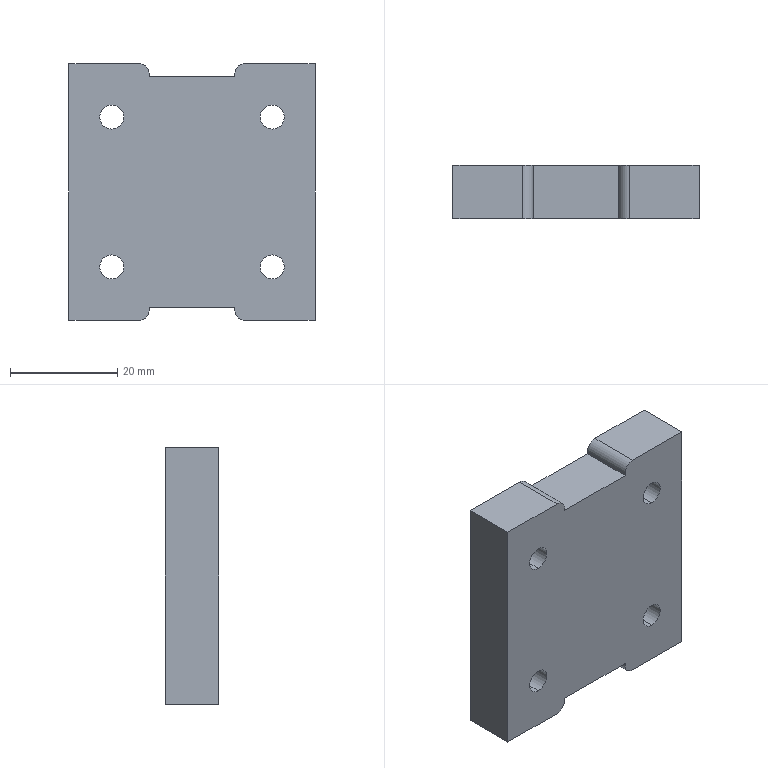Part | SolidWorks | features ICE 2, Extrusion 1, Fillet 1, HoleWzd 1 | 1 solid | 49 faces | box 46 x 10 x 48 mm | volume 19482 mm3 | cylinder 22 | plane 19 | cone 8 | commonest cylinder face diameters 4.5 x8 8 x8 4 x4 14 x2
STEP:
#1=CARTESIAN_POINT('',(0.,0.,17.));
#2=VERTEX_POINT('',#1);
#3=CARTESIAN_POINT('',(0.,0.,31.));
#4=VERTEX_POINT('',#3);
#5=CARTESIAN_POINT('',(0.,0.,24.));
#6=DIRECTION('',(0.,1.,0.));
#7=DIRECTION('',(0.,0.,1.));
#8=AXIS2_PLACEMENT_3D('',#5,#6,#7);
#9=CIRCLE('',#8,7.);
#10=EDGE_CURVE('',#2,#4,#9,.T.);
#11=ORIENTED_EDGE('',*,*,#10,.F.);
#12=CARTESIAN_POINT('',(0.,5.,17.));
#13=VERTEX_POINT('',#12);
#14=CARTESIAN_POINT('',(0.,0.,17.));
#15=DIRECTION('',(0.,1.,0.));
#16=VECTOR('',#15,1000.);
#17=LINE('',#14,#16);
#18=EDGE_CURVE('',#2,#13,#17,.T.);
#19=ORIENTED_EDGE('',*,*,#18,.T.);
#20=CARTESIAN_POINT('',(0.,5.,31.));
#21=VERTEX_POINT('',#20);
#22=CARTESIAN_POINT('',(0.,5.,24.));
#23=DIRECTION('',(0.,1.,0.));
#24=DIRECTION('',(0.,0.,1.));
#25=AXIS2_PLACEMENT_3D('',#22,#23,#24);
#26=CIRCLE('',#25,7.);
#27=EDGE_CURVE('',#13,#21,#26,.T.);
#28=ORIENTED_EDGE('',*,*,#27,.T.);
#29=CARTESIAN_POINT('',(0.,0.,31.));
#30=DIRECTION('',(0.,1.,0.));
#31=VECTOR('',#30,1000.);
#32=LINE('',#29,#31);
#33=EDGE_CURVE('',#4,#21,#32,.T.);
#34=ORIENTED_EDGE('',*,*,#33,.F.);
#35=EDGE_LOOP('',(#11,#19,#28,#34));
#36=FACE_OUTER_BOUND('',#35,.T.);
#37=CARTESIAN_POINT('',(0.,0.,24.));
#38=DIRECTION('',(0.,1.,0.));
#39=DIRECTION('',(0.,0.,1.));
#40=AXIS2_PLACEMENT_3D('',#37,#38,#39);
#41=CYLINDRICAL_SURFACE('',#40,7.);
#42=ADVANCED_FACE('',(#36),#41,.F.);
#43=CARTESIAN_POINT('',(-15.,4.975,6.));
#44=VERTEX_POINT('',#43);
#45=CARTESIAN_POINT('',(-15.,4.975,14.));
#46=VERTEX_POINT('',#45);
#47=CARTESIAN_POINT('',(-15.,4.975,10.));
#48=DIRECTION('',(0.,1.,0.));
#49=DIRECTION('',(0.,0.,1.));
#50=AXIS2_PLACEMENT_3D('',#47,#48,#49);
#51=CIRCLE('',#50,4.);
#52=EDGE_CURVE('',#44,#46,#51,.T.);
#53=ORIENTED_EDGE('',*,*,#52,.F.);
#54=CARTESIAN_POINT('',(-15.,5.,5.975));
#55=VERTEX_POINT('',#54);
#56=CARTESIAN_POINT('',(-15.,5.,5.975));
#57=DIRECTION('',(0.,0.7071,-0.7071));
#58=VECTOR('',#57,1000.);
#59=LINE('',#56,#58);
#60=EDGE_CURVE('',#44,#55,#59,.T.);
#61=ORIENTED_EDGE('',*,*,#60,.T.);
#62=CARTESIAN_POINT('',(-15.,5.,14.025));
#63=VERTEX_POINT('',#62);
#64=CARTESIAN_POINT('',(-15.,5.,10.));
#65=DIRECTION('',(0.,1.,0.));
#66=DIRECTION('',(0.,0.,1.));
#67=AXIS2_PLACEMENT_3D('',#64,#65,#66);
#68=CIRCLE('',#67,4.025);
#69=EDGE_CURVE('',#55,#63,#68,.T.);
#70=ORIENTED_EDGE('',*,*,#69,.T.);
#71=CARTESIAN_POINT('',(-15.,5.,14.025));
#72=DIRECTION('',(0.,0.7071,0.7071));
#73=VECTOR('',#72,1000.);
#74=LINE('',#71,#73);
#75=EDGE_CURVE('',#46,#63,#74,.T.);
#76=ORIENTED_EDGE('',*,*,#75,.F.);
#77=EDGE_LOOP('',(#53,#61,#70,#76));
#78=FACE_OUTER_BOUND('',#77,.T.);
#79=CARTESIAN_POINT('',(-15.,5.,10.));
#80=DIRECTION('',(0.,1.,0.));
#81=DIRECTION('',(0.,0.,1.));
#82=AXIS2_PLACEMENT_3D('',#79,#80,#81);
#83=CONICAL_SURFACE('',#82,4.025,0.7854);
#84=ADVANCED_FACE('',(#78),#83,.F.);
#85=CARTESIAN_POINT('',(-15.,2.4,6.));
#86=VERTEX_POINT('',#85);
#87=CARTESIAN_POINT('',(-15.,2.4,14.));
#88=VERTEX_POINT('',#87);
#89=CARTESIAN_POINT('',(-15.,2.4,10.));
#90=DIRECTION('',(0.,1.,0.));
#91=DIRECTION('',(0.,0.,1.));
#92=AXIS2_PLACEMENT_3D('',#89,#90,#91);
#93=CIRCLE('',#92,4.);
#94=EDGE_CURVE('',#86,#88,#93,.T.);
#95=ORIENTED_EDGE('',*,*,#94,.F.);
#96=CARTESIAN_POINT('',(-15.,5.,6.));
#97=DIRECTION('',(0.,1.,0.));
#98=VECTOR('',#97,1000.);
#99=LINE('',#96,#98);
#100=EDGE_CURVE('',#86,#44,#99,.T.);
#101=ORIENTED_EDGE('',*,*,#100,.T.);
#102=ORIENTED_EDGE('',*,*,#52,.T.);
#103=CARTESIAN_POINT('',(-15.,5.,14.));
#104=DIRECTION('',(0.,1.,0.));
#105=VECTOR('',#104,1000.);
#106=LINE('',#103,#105);
#107=EDGE_CURVE('',#88,#46,#106,.T.);
#108=ORIENTED_EDGE('',*,*,#107,.F.);
#109=EDGE_LOOP('',(#95,#101,#102,#108));
#110=FACE_OUTER_BOUND('',#109,.T.);
#111=CARTESIAN_POINT('',(-15.,5.,10.));
#112=DIRECTION('',(0.,1.,0.));
#113=DIRECTION('',(0.,0.,1.));
#114=AXIS2_PLACEMENT_3D('',#111,#112,#113);
#115=CYLINDRICAL_SURFACE('',#114,4.);
#116=ADVANCED_FACE('',(#110),#115,.F.);
#117=CARTESIAN_POINT('',(-15.,-5.,7.75));
#118=VERTEX_POINT('',#117);
#119=CARTESIAN_POINT('',(-15.,-5.,12.25));
#120=VERTEX_POINT('',#119);
#121=CARTESIAN_POINT('',(-15.,-5.,10.));
#122=DIRECTION('',(0.,1.,0.));
#123=DIRECTION('',(0.,0.,1.));
#124=AXIS2_PLACEMENT_3D('',#121,#122,#123);
#125=CIRCLE('',#124,2.25);
#126=EDGE_CURVE('',#118,#120,#125,.T.);
#127=ORIENTED_EDGE('',*,*,#126,.F.);
#128=CARTESIAN_POINT('',(-15.,2.4,7.75));
#129=VERTEX_POINT('',#128);
#130=CARTESIAN_POINT('',(-15.,5.,7.75));
#131=DIRECTION('',(0.,1.,0.));
#132=VECTOR('',#131,1000.);
#133=LINE('',#130,#132);
#134=EDGE_CURVE('',#118,#129,#133,.T.);
#135=ORIENTED_EDGE('',*,*,#134,.T.);
#136=CARTESIAN_POINT('',(-15.,2.4,12.25));
#137=VERTEX_POINT('',#136);
#138=CARTESIAN_POINT('',(-15.,2.4,10.));
#139=DIRECTION('',(0.,1.,0.));
#140=DIRECTION('',(0.,0.,1.));
#141=AXIS2_PLACEMENT_3D('',#138,#139,#140);
#142=CIRCLE('',#141,2.25);
#143=EDGE_CURVE('',#129,#137,#142,.T.);
#144=ORIENTED_EDGE('',*,*,#143,.T.);
#145=CARTESIAN_POINT('',(-15.,5.,12.25));
#146=DIRECTION('',(0.,1.,0.));
#147=VECTOR('',#146,1000.);
#148=LINE('',#145,#147);
#149=EDGE_CURVE('',#120,#137,#148,.T.);
#150=ORIENTED_EDGE('',*,*,#149,.F.);
#151=EDGE_LOOP('',(#127,#135,#144,#150));
#152=FACE_OUTER_BOUND('',#151,.T.);
#153=CARTESIAN_POINT('',(-15.,5.,10.));
#154=DIRECTION('',(0.,1.,0.));
#155=DIRECTION('',(0.,0.,1.));
#156=AXIS2_PLACEMENT_3D('',#153,#154,#155);
#157=CYLINDRICAL_SURFACE('',#156,2.25);
#158=ADVANCED_FACE('',(#152),#157,.F.);
#159=CARTESIAN_POINT('',(-15.,4.975,34.));
#160=VERTEX_POINT('',#159);
#161=CARTESIAN_POINT('',(-15.,4.975,42.));
#162=VERTEX_POINT('',#161);
#163=CARTESIAN_POINT('',(-15.,4.975,38.));
#164=DIRECTION('',(0.,1.,0.));
#165=DIRECTION('',(0.,0.,1.));
#166=AXIS2_PLACEMENT_3D('',#163,#164,#165);
#167=CIRCLE('',#166,4.);
#168=EDGE_CURVE('',#160,#162,#167,.T.);
#169=ORIENTED_EDGE('',*,*,#168,.F.);
#170=CARTESIAN_POINT('',(-15.,5.,33.975));
#171=VERTEX_POINT('',#170);
#172=CARTESIAN_POINT('',(-15.,5.,33.975));
#173=DIRECTION('',(0.,0.7071,-0.7071));
#174=VECTOR('',#173,1000.);
#175=LINE('',#172,#174);
#176=EDGE_CURVE('',#160,#171,#175,.T.);
#177=ORIENTED_EDGE('',*,*,#176,.T.);
#178=CARTESIAN_POINT('',(-15.,5.,42.025));
#179=VERTEX_POINT('',#178);
#180=CARTESIAN_POINT('',(-15.,5.,38.));
#181=DIRECTION('',(0.,1.,0.));
#182=DIRECTION('',(0.,0.,1.));
#183=AXIS2_PLACEMENT_3D('',#180,#181,#182);
#184=CIRCLE('',#183,4.025);
#185=EDGE_CURVE('',#171,#179,#184,.T.);
#186=ORIENTED_EDGE('',*,*,#185,.T.);
#187=CARTESIAN_POINT('',(-15.,5.,42.025));
#188=DIRECTION('',(0.,0.7071,0.7071));
#189=VECTOR('',#188,1000.);
#190=LINE('',#187,#189);
#191=EDGE_CURVE('',#162,#179,#190,.T.);
#192=ORIENTED_EDGE('',*,*,#191,.F.);
#193=EDGE_LOOP('',(#169,#177,#186,#192));
#194=FACE_OUTER_BOUND('',#193,.T.);
#195=CARTESIAN_POINT('',(-15.,5.,38.));
#196=DIRECTION('',(0.,1.,0.));
#197=DIRECTION('',(0.,0.,1.));
#198=AXIS2_PLACEMENT_3D('',#195,#196,#197);
#199=CONICAL_SURFACE('',#198,4.025,0.7854);
#200=ADVANCED_FACE('',(#194),#199,.F.);
#201=CARTESIAN_POINT('',(-15.,2.4,34.));
#202=VERTEX_POINT('',#201);
#203=CARTESIAN_POINT('',(-15.,2.4,42.));
#204=VERTEX_POINT('',#203);
#205=CARTESIAN_POINT('',(-15.,2.4,38.));
#206=DIRECTION('',(0.,1.,0.));
#207=DIRECTION('',(0.,0.,1.));
#208=AXIS2_PLACEMENT_3D('',#205,#206,#207);
#209=CIRCLE('',#208,4.);
#210=EDGE_CURVE('',#202,#204,#209,.T.);
#211=ORIENTED_EDGE('',*,*,#210,.F.);
#212=CARTESIAN_POINT('',(-15.,5.,34.));
#213=DIRECTION('',(0.,1.,0.));
#214=VECTOR('',#213,1000.);
#215=LINE('',#212,#214);
#216=EDGE_CURVE('',#202,#160,#215,.T.);
#217=ORIENTED_EDGE('',*,*,#216,.T.);
#218=ORIENTED_EDGE('',*,*,#168,.T.);
#219=CARTESIAN_POINT('',(-15.,5.,42.));
#220=DIRECTION('',(0.,1.,0.));
#221=VECTOR('',#220,1000.);
#222=LINE('',#219,#221);
#223=EDGE_CURVE('',#204,#162,#222,.T.);
#224=ORIENTED_EDGE('',*,*,#223,.F.);
#225=EDGE_LOOP('',(#211,#217,#218,#224));
#226=FACE_OUTER_BOUND('',#225,.T.);
#227=CARTESIAN_POINT('',(-15.,5.,38.));
#228=DIRECTION('',(0.,1.,0.));
#229=DIRECTION('',(0.,0.,1.));
#230=AXIS2_PLACEMENT_3D('',#227,#228,#229);
#231=CYLINDRICAL_SURFACE('',#230,4.);
#232=ADVANCED_FACE('',(#226),#231,.F.);
#233=CARTESIAN_POINT('',(-15.,-5.,35.75));
#234=VERTEX_POINT('',#233);
#235=CARTESIAN_POINT('',(-15.,-5.,40.25));
#236=VERTEX_POINT('',#235);
#237=CARTESIAN_POINT('',(-15.,-5.,38.));
#238=DIRECTION('',(0.,1.,0.));
#239=DIRECTION('',(0.,0.,1.));
#240=AXIS2_PLACEMENT_3D('',#237,#238,#239);
#241=CIRCLE('',#240,2.25);
#242=EDGE_CURVE('',#234,#236,#241,.T.);
#243=ORIENTED_EDGE('',*,*,#242,.F.);
#244=CARTESIAN_POINT('',(-15.,2.4,35.75));
#245=VERTEX_POINT('',#244);
#246=CARTESIAN_POINT('',(-15.,5.,35.75));
#247=DIRECTION('',(0.,1.,0.));
#248=VECTOR('',#247,1000.);
#249=LINE('',#246,#248);
#250=EDGE_CURVE('',#234,#245,#249,.T.);
#251=ORIENTED_EDGE('',*,*,#250,.T.);
#252=CARTESIAN_POINT('',(-15.,2.4,40.25));
#253=VERTEX_POINT('',#252);
#254=CARTESIAN_POINT('',(-15.,2.4,38.));
#255=DIRECTION('',(0.,1.,0.));
#256=DIRECTION('',(0.,0.,1.));
#257=AXIS2_PLACEMENT_3D('',#254,#255,#256);
#258=CIRCLE('',#257,2.25);
#259=EDGE_CURVE('',#245,#253,#258,.T.);
#260=ORIENTED_EDGE('',*,*,#259,.T.);
#261=CARTESIAN_POINT('',(-15.,5.,40.25));
#262=DIRECTION('',(0.,1.,0.));
#263=VECTOR('',#262,1000.);
#264=LINE('',#261,#263);
#265=EDGE_CURVE('',#236,#253,#264,.T.);
#266=ORIENTED_EDGE('',*,*,#265,.F.);
#267=EDGE_LOOP('',(#243,#251,#260,#266));
#268=FACE_OUTER_BOUND('',#267,.T.);
#269=CARTESIAN_POINT('',(-15.,5.,38.));
#270=DIRECTION('',(0.,1.,0.));
#271=DIRECTION('',(0.,0.,1.));
#272=AXIS2_PLACEMENT_3D('',#269,#270,#271);
#273=CYLINDRICAL_SURFACE('',#272,2.25);
#274=ADVANCED_FACE('',(#268),#273,.F.);
#275=CARTESIAN_POINT('',(15.,4.975,34.));
#276=VERTEX_POINT('',#275);
#277=CARTESIAN_POINT('',(15.,4.975,42.));
#278=VERTEX_POINT('',#277);
#279=CARTESIAN_POINT('',(15.,4.975,38.));
#280=DIRECTION('',(0.,1.,0.));
#281=DIRECTION('',(0.,0.,1.));
#282=AXIS2_PLACEMENT_3D('',#279,#280,#281);
#283=CIRCLE('',#282,4.);
#284=EDGE_CURVE('',#276,#278,#283,.T.);
#285=ORIENTED_EDGE('',*,*,#284,.F.);
#286=CARTESIAN_POINT('',(15.,5.,33.975));
#287=VERTEX_POINT('',#286);
#288=CARTESIAN_POINT('',(15.,5.,33.975));
#289=DIRECTION('',(0.,0.7071,-0.7071));
#290=VECTOR('',#289,1000.);
#291=LINE('',#288,#290);
#292=EDGE_CURVE('',#276,#287,#291,.T.);
#293=ORIENTED_EDGE('',*,*,#292,.T.);
#294=CARTESIAN_POINT('',(15.,5.,42.025));
#295=VERTEX_POINT('',#294);
#296=CARTESIAN_POINT('',(15.,5.,38.));
#297=DIRECTION('',(0.,1.,0.));
#298=DIRECTION('',(0.,0.,1.));
#299=AXIS2_PLACEMENT_3D('',#296,#297,#298);
#300=CIRCLE('',#299,4.025);
#301=EDGE_CURVE('',#287,#295,#300,.T.);
#302=ORIENTED_EDGE('',*,*,#301,.T.);
#303=CARTESIAN_POINT('',(15.,5.,42.025));
#304=DIRECTION('',(0.,0.7071,0.7071));
#305=VECTOR('',#304,1000.);
#306=LINE('',#303,#305);
#307=EDGE_CURVE('',#278,#295,#306,.T.);
#308=ORIENTED_EDGE('',*,*,#307,.F.);
#309=EDGE_LOOP('',(#285,#293,#302,#308));
#310=FACE_OUTER_BOUND('',#309,.T.);
#311=CARTESIAN_POINT('',(15.,5.,38.));
#312=DIRECTION('',(0.,1.,0.));
#313=DIRECTION('',(0.,0.,1.));
#314=AXIS2_PLACEMENT_3D('',#311,#312,#313);
#315=CONICAL_SURFACE('',#314,4.025,0.7854);
#316=ADVANCED_FACE('',(#310),#315,.F.);
#317=CARTESIAN_POINT('',(15.,2.4,34.));
#318=VERTEX_POINT('',#317);
#319=CARTESIAN_POINT('',(15.,2.4,42.));
#320=VERTEX_POINT('',#319);
#321=CARTESIAN_POINT('',(15.,2.4,38.));
#322=DIRECTION('',(0.,1.,0.));
#323=DIRECTION('',(0.,0.,1.));
#324=AXIS2_PLACEMENT_3D('',#321,#322,#323);
#325=CIRCLE('',#324,4.);
#326=EDGE_CURVE('',#318,#320,#325,.T.);
#327=ORIENTED_EDGE('',*,*,#326,.F.);
#328=CARTESIAN_POINT('',(15.,5.,34.));
#329=DIRECTION('',(0.,1.,0.));
#330=VECTOR('',#329,1000.);
#331=LINE('',#328,#330);
#332=EDGE_CURVE('',#318,#276,#331,.T.);
#333=ORIENTED_EDGE('',*,*,#332,.T.);
#334=ORIENTED_EDGE('',*,*,#284,.T.);
#335=CARTESIAN_POINT('',(15.,5.,42.));
#336=DIRECTION('',(0.,1.,0.));
#337=VECTOR('',#336,1000.);
#338=LINE('',#335,#337);
#339=EDGE_CURVE('',#320,#278,#338,.T.);
#340=ORIENTED_EDGE('',*,*,#339,.F.);
#341=EDGE_LOOP('',(#327,#333,#334,#340));
#342=FACE_OUTER_BOUND('',#341,.T.);
#343=CARTESIAN_POINT('',(15.,5.,38.));
#344=DIRECTION('',(0.,1.,0.));
#345=DIRECTION('',(0.,0.,1.));
#346=AXIS2_PLACEMENT_3D('',#343,#344,#345);
#347=CYLINDRICAL_SURFACE('',#346,4.);
#348=ADVANCED_FACE('',(#342),#347,.F.);
#349=CARTESIAN_POINT('',(15.,-5.,35.75));
#350=VERTEX_POINT('',#349);
#351=CARTESIAN_POINT('',(15.,-5.,40.25));
#352=VERTEX_POINT('',#351);
#353=CARTESIAN_POINT('',(15.,-5.,38.));
#354=DIRECTION('',(0.,1.,0.));
#355=DIRECTION('',(0.,0.,1.));
#356=AXIS2_PLACEMENT_3D('',#353,#354,#355);
#357=CIRCLE('',#356,2.25);
#358=EDGE_CURVE('',#350,#352,#357,.T.);
#359=ORIENTED_EDGE('',*,*,#358,.F.);
#360=CARTESIAN_POINT('',(15.,2.4,35.75));
#361=VERTEX_POINT('',#360);
#362=CARTESIAN_POINT('',(15.,5.,35.75));
#363=DIRECTION('',(0.,1.,0.));
#364=VECTOR('',#363,1000.);
#365=LINE('',#362,#364);
#366=EDGE_CURVE('',#350,#361,#365,.T.);
#367=ORIENTED_EDGE('',*,*,#366,.T.);
#368=CARTESIAN_POINT('',(15.,2.4,40.25));
#369=VERTEX_POINT('',#368);
#370=CARTESIAN_POINT('',(15.,2.4,38.));
#371=DIRECTION('',(0.,1.,0.));
#372=DIRECTION('',(0.,0.,1.));
#373=AXIS2_PLACEMENT_3D('',#370,#371,#372);
#374=CIRCLE('',#373,2.25);
#375=EDGE_CURVE('',#361,#369,#374,.T.);
#376=ORIENTED_EDGE('',*,*,#375,.T.);
#377=CARTESIAN_POINT('',(15.,5.,40.25));
#378=DIRECTION('',(0.,1.,0.));
#379=VECTOR('',#378,1000.);
#380=LINE('',#377,#379);
#381=EDGE_CURVE('',#352,#369,#380,.T.);
#382=ORIENTED_EDGE('',*,*,#381,.F.);
#383=EDGE_LOOP('',(#359,#367,#376,#382));
#384=FACE_OUTER_BOUND('',#383,.T.);
#385=CARTESIAN_POINT('',(15.,5.,38.));
#386=DIRECTION('',(0.,1.,0.));
#387=DIRECTION('',(0.,0.,1.));
#388=AXIS2_PLACEMENT_3D('',#385,#386,#387);
#389=CYLINDRICAL_SURFACE('',#388,2.25);
#390=ADVANCED_FACE('',(#384),#389,.F.);
#391=CARTESIAN_POINT('',(15.,4.975,6.));
#392=VERTEX_POINT('',#391);
#393=CARTESIAN_POINT('',(15.,4.975,14.));
#394=VERTEX_POINT('',#393);
#395=CARTESIAN_POINT('',(15.,4.975,10.));
#396=DIRECTION('',(0.,1.,0.));
#397=DIRECTION('',(0.,0.,1.));
#398=AXIS2_PLACEMENT_3D('',#395,#396,#397);
#399=CIRCLE('',#398,4.);
#400=EDGE_CURVE('',#392,#394,#399,.T.);
#401=ORIENTED_EDGE('',*,*,#400,.F.);
#402=CARTESIAN_POINT('',(15.,5.,5.975));
#403=VERTEX_POINT('',#402);
#404=CARTESIAN_POINT('',(15.,5.,5.975));
#405=DIRECTION('',(0.,0.7071,-0.7071));
#406=VECTOR('',#405,1000.);
#407=LINE('',#404,#406);
#408=EDGE_CURVE('',#392,#403,#407,.T.);
#409=ORIENTED_EDGE('',*,*,#408,.T.);
#410=CARTESIAN_POINT('',(15.,5.,14.025));
#411=VERTEX_POINT('',#410);
#412=CARTESIAN_POINT('',(15.,5.,10.));
#413=DIRECTION('',(0.,1.,0.));
#414=DIRECTION('',(0.,0.,1.));
#415=AXIS2_PLACEMENT_3D('',#412,#413,#414);
#416=CIRCLE('',#415,4.025);
#417=EDGE_CURVE('',#403,#411,#416,.T.);
#418=ORIENTED_EDGE('',*,*,#417,.T.);
#419=CARTESIAN_POINT('',(15.,5.,14.025));
#420=DIRECTION('',(0.,0.7071,0.7071));
#421=VECTOR('',#420,1000.);
#422=LINE('',#419,#421);
#423=EDGE_CURVE('',#394,#411,#422,.T.);
#424=ORIENTED_EDGE('',*,*,#423,.F.);
#425=EDGE_LOOP('',(#401,#409,#418,#424));
#426=FACE_OUTER_BOUND('',#425,.T.);
#427=CARTESIAN_POINT('',(15.,5.,10.));
#428=DIRECTION('',(0.,1.,0.));
#429=DIRECTION('',(0.,0.,1.));
#430=AXIS2_PLACEMENT_3D('',#427,#428,#429);
#431=CONICAL_SURFACE('',#430,4.025,0.7854);
#432=ADVANCED_FACE('',(#426),#431,.F.);
#433=CARTESIAN_POINT('',(15.,2.4,6.));
#434=VERTEX_POINT('',#433);
#435=CARTESIAN_POINT('',(15.,2.4,14.));
#436=VERTEX_POINT('',#435);
#437=CARTESIAN_POINT('',(15.,2.4,10.));
#438=DIRECTION('',(0.,1.,0.));
#439=DIRECTION('',(0.,0.,1.));
#440=AXIS2_PLACEMENT_3D('',#437,#438,#439);
#441=CIRCLE('',#440,4.);
#442=EDGE_CURVE('',#434,#436,#441,.T.);
#443=ORIENTED_EDGE('',*,*,#442,.F.);
#444=CARTESIAN_POINT('',(15.,5.,6.));
#445=DIRECTION('',(0.,1.,0.));
#446=VECTOR('',#445,1000.);
#447=LINE('',#444,#446);
#448=EDGE_CURVE('',#434,#392,#447,.T.);
#449=ORIENTED_EDGE('',*,*,#448,.T.);
#450=ORIENTED_EDGE('',*,*,#400,.T.);
#451=CARTESIAN_POINT('',(15.,5.,14.));
#452=DIRECTION('',(0.,1.,0.));
#453=VECTOR('',#452,1000.);
#454=LINE('',#451,#453);
#455=EDGE_CURVE('',#436,#394,#454,.T.);
#456=ORIENTED_EDGE('',*,*,#455,.F.);
#457=EDGE_LOOP('',(#443,#449,#450,#456));
#458=FACE_OUTER_BOUND('',#457,.T.);
#459=CARTESIAN_POINT('',(15.,5.,10.));
#460=DIRECTION('',(0.,1.,0.));
#461=DIRECTION('',(0.,0.,1.));
#462=AXIS2_PLACEMENT_3D('',#459,#460,#461);
#463=CYLINDRICAL_SURFACE('',#462,4.);
#464=ADVANCED_FACE('',(#458),#463,.F.);
#465=CARTESIAN_POINT('',(15.,-5.,7.75));
#466=VERTEX_POINT('',#465);
#467=CARTESIAN_POINT('',(15.,-5.,12.25));
#468=VERTEX_POINT('',#467);
#469=CARTESIAN_POINT('',(15.,-5.,10.));
#470=DIRECTION('',(0.,1.,0.));
#471=DIRECTION('',(0.,0.,1.));
#472=AXIS2_PLACEMENT_3D('',#469,#470,#471);
#473=CIRCLE('',#472,2.25);
#474=EDGE_CURVE('',#466,#468,#473,.T.);
#475=ORIENTED_EDGE('',*,*,#474,.F.);
#476=CARTESIAN_POINT('',(15.,2.4,7.75));
#477=VERTEX_POINT('',#476);
#478=CARTESIAN_POINT('',(15.,5.,7.75));
#479=DIRECTION('',(0.,1.,0.));
#480=VECTOR('',#479,1000.);
#481=LINE('',#478,#480);
#482=EDGE_CURVE('',#466,#477,#481,.T.);
#483=ORIENTED_EDGE('',*,*,#482,.T.);
#484=CARTESIAN_POINT('',(15.,2.4,12.25));
#485=VERTEX_POINT('',#484);
#486=CARTESIAN_POINT('',(15.,2.4,10.));
#487=DIRECTION('',(0.,1.,0.));
#488=DIRECTION('',(0.,0.,1.));
#489=AXIS2_PLACEMENT_3D('',#486,#487,#488);
#490=CIRCLE('',#489,2.25);
#491=EDGE_CURVE('',#477,#485,#490,.T.);
#492=ORIENTED_EDGE('',*,*,#491,.T.);
#493=CARTESIAN_POINT('',(15.,5.,12.25));
#494=DIRECTION('',(0.,1.,0.));
#495=VECTOR('',#494,1000.);
#496=LINE('',#493,#495);
#497=EDGE_CURVE('',#468,#485,#496,.T.);
#498=ORIENTED_EDGE('',*,*,#497,.F.);
#499=EDGE_LOOP('',(#475,#483,#492,#498));
#500=FACE_OUTER_BOUND('',#499,.T.);
#501=CARTESIAN_POINT('',(15.,5.,10.));
#502=DIRECTION('',(0.,1.,0.));
#503=DIRECTION('',(0.,0.,1.));
#504=AXIS2_PLACEMENT_3D('',#501,#502,#503);
#505=CYLINDRICAL_SURFACE('',#504,2.25);
#506=ADVANCED_FACE('',(#500),#505,.F.);
#507=CARTESIAN_POINT('',(-23.,-5.,48.));
#508=VERTEX_POINT('',#507);
#509=CARTESIAN_POINT('',(-10.,-5.,48.));
#510=VERTEX_POINT('',#509);
#511=CARTESIAN_POINT('',(-23.,-5.,48.));
#512=DIRECTION('',(1.,0.,0.));
#513=VECTOR('',#512,1000.);
#514=LINE('',#511,#513);
#515=EDGE_CURVE('',#508,#510,#514,.T.);
#516=ORIENTED_EDGE('',*,*,#515,.T.);
#517=CARTESIAN_POINT('',(-10.,5.,48.));
#518=VERTEX_POINT('',#517);
#519=CARTESIAN_POINT('',(-10.,5.,48.));
#520=DIRECTION('',(0.,1.,0.));
#521=VECTOR('',#520,1000.);
#522=LINE('',#519,#521);
#523=EDGE_CURVE('',#510,#518,#522,.T.);
#524=ORIENTED_EDGE('',*,*,#523,.T.);
#525=CARTESIAN_POINT('',(-23.,5.,48.));
#526=VERTEX_POINT('',#525);
#527=CARTESIAN_POINT('',(-23.,5.,48.));
#528=DIRECTION('',(-1.,0.,0.));
#529=VECTOR('',#528,1000.);
#530=LINE('',#527,#529);
#531=EDGE_CURVE('',#518,#526,#530,.T.);
#532=ORIENTED_EDGE('',*,*,#531,.T.);
#533=CARTESIAN_POINT('',(-23.,5.,48.));
#534=DIRECTION('',(0.,-1.,0.));
#535=VECTOR('',#534,1000.);
#536=LINE('',#533,#535);
#537=EDGE_CURVE('',#526,#508,#536,.T.);
#538=ORIENTED_EDGE('',*,*,#537,.T.);
#539=EDGE_LOOP('',(#516,#524,#532,#538));
#540=FACE_OUTER_BOUND('',#539,.T.);
#541=CARTESIAN_POINT('',(0.,0.,48.));
#542=DIRECTION('',(0.,0.,1.));
#543=DIRECTION('',(1.,0.,0.));
#544=AXIS2_PLACEMENT_3D('',#541,#542,#543);
#545=PLANE('',#544);
#546=ADVANCED_FACE('',(#540),#545,.T.);
#547=CARTESIAN_POINT('',(10.,-5.,0.));
#548=VERTEX_POINT('',#547);
#549=CARTESIAN_POINT('',(23.,-5.,0.));
#550=VERTEX_POINT('',#549);
#551=CARTESIAN_POINT('',(-23.,-5.,0.));
#552=DIRECTION('',(1.,0.,0.));
#553=VECTOR('',#552,1000.);
#554=LINE('',#551,#553);
#555=EDGE_CURVE('',#548,#550,#554,.T.);
#556=ORIENTED_EDGE('',*,*,#555,.F.);
#557=CARTESIAN_POINT('',(10.,5.,0.));
#558=VERTEX_POINT('',#557);
#559=CARTESIAN_POINT('',(10.,0.,0.));
#560=DIRECTION('',(0.,1.,0.));
#561=VECTOR('',#560,1000.);
#562=LINE('',#559,#561);
#563=EDGE_CURVE('',#548,#558,#562,.T.);
#564=ORIENTED_EDGE('',*,*,#563,.T.);
#565=CARTESIAN_POINT('',(23.,5.,0.));
#566=VERTEX_POINT('',#565);
#567=CARTESIAN_POINT('',(-23.,5.,0.));
#568=DIRECTION('',(-1.,0.,0.));
#569=VECTOR('',#568,1000.);
#570=LINE('',#567,#569);
#571=EDGE_CURVE('',#566,#558,#570,.T.);
#572=ORIENTED_EDGE('',*,*,#571,.F.);
#573=CARTESIAN_POINT('',(23.,5.,0.));
#574=DIRECTION('',(0.,1.,0.));
#575=VECTOR('',#574,1000.);
#576=LINE('',#573,#575);
#577=EDGE_CURVE('',#550,#566,#576,.T.);
#578=ORIENTED_EDGE('',*,*,#577,.F.);
#579=EDGE_LOOP('',(#556,#564,#572,#578));
#580=FACE_OUTER_BOUND('',#579,.T.);
#581=CARTESIAN_POINT('',(0.,0.,0.));
#582=DIRECTION('',(0.,0.,1.));
#583=DIRECTION('',(1.,0.,0.));
#584=AXIS2_PLACEMENT_3D('',#581,#582,#583);
#585=PLANE('',#584);
#586=ADVANCED_FACE('',(#580),#585,.F.);
#587=ORIENTED_EDGE('',*,*,#577,.T.);
#588=CARTESIAN_POINT('',(23.,5.,48.));
#589=VERTEX_POINT('',#588);
#590=CARTESIAN_POINT('',(23.,5.,48.));
#591=DIRECTION('',(0.,0.,-1.));
#592=VECTOR('',#591,1000.);
#593=LINE('',#590,#592);
#594=EDGE_CURVE('',#589,#566,#593,.T.);
#595=ORIENTED_EDGE('',*,*,#594,.F.);
#596=CARTESIAN_POINT('',(23.,-5.,48.));
#597=VERTEX_POINT('',#596);
#598=CARTESIAN_POINT('',(23.,5.,48.));
#599=DIRECTION('',(0.,1.,0.));
#600=VECTOR('',#599,1000.);
#601=LINE('',#598,#600);
#602=EDGE_CURVE('',#597,#589,#601,.T.);
#603=ORIENTED_EDGE('',*,*,#602,.F.);
#604=CARTESIAN_POINT('',(23.,-5.,48.));
#605=DIRECTION('',(0.,0.,-1.));
#606=VECTOR('',#605,1000.);
#607=LINE('',#604,#606);
#608=EDGE_CURVE('',#597,#550,#607,.T.);
#609=ORIENTED_EDGE('',*,*,#608,.T.);
#610=EDGE_LOOP('',(#587,#595,#603,#609));
#611=FACE_OUTER_BOUND('',#610,.T.);
#612=CARTESIAN_POINT('',(23.,5.,48.));
#613=DIRECTION('',(-1.,0.,0.));
#614=DIRECTION('',(0.,0.,1.));
#615=AXIS2_PLACEMENT_3D('',#612,#613,#614);
#616=PLANE('',#615);
#617=ADVANCED_FACE('',(#611),#616,.F.);
#618=CARTESIAN_POINT('',(0.,5.,24.));
#619=DIRECTION('',(0.,1.,0.));
#620=DIRECTION('',(0.,0.,1.));
#621=AXIS2_PLACEMENT_3D('',#618,#619,#620);
#622=CIRCLE('',#621,7.);
#623=EDGE_CURVE('',#21,#13,#622,.T.);
#624=ORIENTED_EDGE('',*,*,#623,.F.);
#625=ORIENTED_EDGE('',*,*,#27,.F.);
#626=EDGE_LOOP('',(#624,#625));
#627=FACE_BOUND('',#626,.T.);
#628=CARTESIAN_POINT('',(-15.,5.,10.));
#629=DIRECTION('',(0.,1.,0.));
#630=DIRECTION('',(0.,0.,1.));
#631=AXIS2_PLACEMENT_3D('',#628,#629,#630);
#632=CIRCLE('',#631,4.025);
#633=EDGE_CURVE('',#63,#55,#632,.T.);
#634=ORIENTED_EDGE('',*,*,#633,.F.);
#635=ORIENTED_EDGE('',*,*,#69,.F.);
#636=EDGE_LOOP('',(#634,#635));
#637=FACE_BOUND('',#636,.T.);
#638=CARTESIAN_POINT('',(-15.,5.,38.));
#639=DIRECTION('',(0.,1.,0.));
#640=DIRECTION('',(0.,0.,1.));
#641=AXIS2_PLACEMENT_3D('',#638,#639,#640);
#642=CIRCLE('',#641,4.025);
#643=EDGE_CURVE('',#179,#171,#642,.T.);
#644=ORIENTED_EDGE('',*,*,#643,.F.);
#645=ORIENTED_EDGE('',*,*,#185,.F.);
#646=EDGE_LOOP('',(#644,#645));
#647=FACE_BOUND('',#646,.T.);
#648=CARTESIAN_POINT('',(15.,5.,38.));
#649=DIRECTION('',(0.,1.,0.));
#650=DIRECTION('',(0.,0.,1.));
#651=AXIS2_PLACEMENT_3D('',#648,#649,#650);
#652=CIRCLE('',#651,4.025);
#653=EDGE_CURVE('',#295,#287,#652,.T.);
#654=ORIENTED_EDGE('',*,*,#653,.F.);
#655=ORIENTED_EDGE('',*,*,#301,.F.);
#656=EDGE_LOOP('',(#654,#655));
#657=FACE_BOUND('',#656,.T.);
#658=CARTESIAN_POINT('',(15.,5.,10.));
#659=DIRECTION('',(0.,1.,0.));
#660=DIRECTION('',(0.,0.,1.));
#661=AXIS2_PLACEMENT_3D('',#658,#659,#660);
#662=CIRCLE('',#661,4.025);
#663=EDGE_CURVE('',#411,#403,#662,.T.);
#664=ORIENTED_EDGE('',*,*,#663,.F.);
#665=ORIENTED_EDGE('',*,*,#417,.F.);
#666=EDGE_LOOP('',(#664,#665));
#667=FACE_BOUND('',#666,.T.);
#668=CARTESIAN_POINT('',(8.,5.,46.));
#669=VERTEX_POINT('',#668);
#670=CARTESIAN_POINT('',(8.,5.,45.5));
#671=VERTEX_POINT('',#670);
#672=CARTESIAN_POINT('',(8.,5.,50.5));
#673=DIRECTION('',(0.,0.,-1.));
#674=VECTOR('',#673,1000.);
#675=LINE('',#672,#674);
#676=EDGE_CURVE('',#669,#671,#675,.T.);
#677=ORIENTED_EDGE('',*,*,#676,.F.);
#678=CARTESIAN_POINT('',(10.,5.,48.));
#679=VERTEX_POINT('',#678);
#680=CARTESIAN_POINT('',(10.,5.,46.));
#681=DIRECTION('',(0.,1.,0.));
#682=DIRECTION('',(0.,0.,-1.));
#683=AXIS2_PLACEMENT_3D('',#680,#681,#682);
#684=CIRCLE('',#683,2.);
#685=EDGE_CURVE('',#669,#679,#684,.T.);
#686=ORIENTED_EDGE('',*,*,#685,.T.);
#687=CARTESIAN_POINT('',(-23.,5.,48.));
#688=DIRECTION('',(-1.,0.,0.));
#689=VECTOR('',#688,1000.);
#690=LINE('',#687,#689);
#691=EDGE_CURVE('',#589,#679,#690,.T.);
#692=ORIENTED_EDGE('',*,*,#691,.F.);
#693=ORIENTED_EDGE('',*,*,#594,.T.);
#694=ORIENTED_EDGE('',*,*,#571,.T.);
#695=CARTESIAN_POINT('',(8.,5.,2.));
#696=VERTEX_POINT('',#695);
#697=CARTESIAN_POINT('',(10.,5.,2.));
#698=DIRECTION('',(0.,1.,0.));
#699=DIRECTION('',(0.,0.,-1.));
#700=AXIS2_PLACEMENT_3D('',#697,#698,#699);
#701=CIRCLE('',#700,2.);
#702=EDGE_CURVE('',#558,#696,#701,.T.);
#703=ORIENTED_EDGE('',*,*,#702,.T.);
#704=CARTESIAN_POINT('',(8.,5.,2.5));
#705=VERTEX_POINT('',#704);
#706=CARTESIAN_POINT('',(8.,5.,-2.5));
#707=DIRECTION('',(0.,0.,-1.));
#708=VECTOR('',#707,1000.);
#709=LINE('',#706,#708);
#710=EDGE_CURVE('',#705,#696,#709,.T.);
#711=ORIENTED_EDGE('',*,*,#710,.F.);
#712=CARTESIAN_POINT('',(-8.,5.,2.5));
#713=VERTEX_POINT('',#712);
#714=CARTESIAN_POINT('',(-8.,5.,2.5));
#715=DIRECTION('',(1.,0.,0.));
#716=VECTOR('',#715,1000.);
#717=LINE('',#714,#716);
#718=EDGE_CURVE('',#713,#705,#717,.T.);
#719=ORIENTED_EDGE('',*,*,#718,.F.);
#720=CARTESIAN_POINT('',(-8.,5.,2.));
#721=VERTEX_POINT('',#720);
#722=CARTESIAN_POINT('',(-8.,5.,-2.5));
#723=DIRECTION('',(0.,0.,1.));
#724=VECTOR('',#723,1000.);
#725=LINE('',#722,#724);
#726=EDGE_CURVE('',#721,#713,#725,.T.);
#727=ORIENTED_EDGE('',*,*,#726,.F.);
#728=CARTESIAN_POINT('',(-10.,5.,0.));
#729=VERTEX_POINT('',#728);
#730=CARTESIAN_POINT('',(-10.,5.,2.));
#731=DIRECTION('',(0.,1.,0.));
#732=DIRECTION('',(0.,0.,-1.));
#733=AXIS2_PLACEMENT_3D('',#730,#731,#732);
#734=CIRCLE('',#733,2.);
#735=EDGE_CURVE('',#721,#729,#734,.T.);
#736=ORIENTED_EDGE('',*,*,#735,.T.);
#737=CARTESIAN_POINT('',(-23.,5.,0.));
#738=VERTEX_POINT('',#737);
#739=CARTESIAN_POINT('',(-23.,5.,0.));
#740=DIRECTION('',(-1.,0.,0.));
#741=VECTOR('',#740,1000.);
#742=LINE('',#739,#741);
#743=EDGE_CURVE('',#729,#738,#742,.T.);
#744=ORIENTED_EDGE('',*,*,#743,.T.);
#745=CARTESIAN_POINT('',(-23.,5.,48.));
#746=DIRECTION('',(0.,0.,-1.));
#747=VECTOR('',#746,1000.);
#748=LINE('',#745,#747);
#749=EDGE_CURVE('',#526,#738,#748,.T.);
#750=ORIENTED_EDGE('',*,*,#749,.F.);
#751=ORIENTED_EDGE('',*,*,#531,.F.);
#752=CARTESIAN_POINT('',(-8.,5.,46.));
#753=VERTEX_POINT('',#752);
#754=CARTESIAN_POINT('',(-10.,5.,46.));
#755=DIRECTION('',(0.,1.,0.));
#756=DIRECTION('',(0.,0.,-1.));
#757=AXIS2_PLACEMENT_3D('',#754,#755,#756);
#758=CIRCLE('',#757,2.);
#759=EDGE_CURVE('',#518,#753,#758,.T.);
#760=ORIENTED_EDGE('',*,*,#759,.T.);
#761=CARTESIAN_POINT('',(-8.,5.,45.5));
#762=VERTEX_POINT('',#761);
#763=CARTESIAN_POINT('',(-8.,5.,50.5));
#764=DIRECTION('',(0.,0.,1.));
#765=VECTOR('',#764,1000.);
#766=LINE('',#763,#765);
#767=EDGE_CURVE('',#762,#753,#766,.T.);
#768=ORIENTED_EDGE('',*,*,#767,.F.);
#769=CARTESIAN_POINT('',(-8.,5.,45.5));
#770=DIRECTION('',(-1.,0.,0.));
#771=VECTOR('',#770,1000.);
#772=LINE('',#769,#771);
#773=EDGE_CURVE('',#671,#762,#772,.T.);
#774=ORIENTED_EDGE('',*,*,#773,.F.);
#775=EDGE_LOOP('',(#677,#686,#692,#693,#694,#703,#711,#719,#727,#736,#744,#750,#751,#760,#768,#774));
#776=FACE_OUTER_BOUND('',#775,.T.);
#777=CARTESIAN_POINT('',(-23.,5.,48.));
#778=DIRECTION('',(0.,-1.,0.));
#779=DIRECTION('',(0.,0.,-1.));
#780=AXIS2_PLACEMENT_3D('',#777,#778,#779);
#781=PLANE('',#780);
#782=ADVANCED_FACE('',(#627,#637,#647,#657,#667,#776),#781,.F.);
#783=CARTESIAN_POINT('',(-23.,-5.,0.));
#784=VERTEX_POINT('',#783);
#785=CARTESIAN_POINT('',(-23.,5.,0.));
#786=DIRECTION('',(0.,-1.,0.));
#787=VECTOR('',#786,1000.);
#788=LINE('',#785,#787);
#789=EDGE_CURVE('',#738,#784,#788,.T.);
#790=ORIENTED_EDGE('',*,*,#789,.T.);
#791=CARTESIAN_POINT('',(-23.,-5.,48.));
#792=DIRECTION('',(0.,0.,-1.));
#793=VECTOR('',#792,1000.);
#794=LINE('',#791,#793);
#795=EDGE_CURVE('',#508,#784,#794,.T.);
#796=ORIENTED_EDGE('',*,*,#795,.F.);
#797=ORIENTED_EDGE('',*,*,#537,.F.);
#798=ORIENTED_EDGE('',*,*,#749,.T.);
#799=EDGE_LOOP('',(#790,#796,#797,#798));
#800=FACE_OUTER_BOUND('',#799,.T.);
#801=CARTESIAN_POINT('',(-23.,5.,48.));
#802=DIRECTION('',(1.,0.,0.));
#803=DIRECTION('',(0.,0.,-1.));
#804=AXIS2_PLACEMENT_3D('',#801,#802,#803);
#805=PLANE('',#804);
#806=ADVANCED_FACE('',(#800),#805,.F.);
#807=CARTESIAN_POINT('',(-15.,-5.,10.));
#808=DIRECTION('',(0.,1.,0.));
#809=DIRECTION('',(0.,0.,1.));
#810=AXIS2_PLACEMENT_3D('',#807,#808,#809);
#811=CIRCLE('',#810,2.25);
#812=EDGE_CURVE('',#120,#118,#811,.T.);
#813=ORIENTED_EDGE('',*,*,#812,.T.);
#814=ORIENTED_EDGE('',*,*,#126,.T.);
#815=EDGE_LOOP('',(#813,#814));
#816=FACE_BOUND('',#815,.T.);
#817=CARTESIAN_POINT('',(-15.,-5.,38.));
#818=DIRECTION('',(0.,1.,0.));
#819=DIRECTION('',(0.,0.,1.));
#820=AXIS2_PLACEMENT_3D('',#817,#818,#819);
#821=CIRCLE('',#820,2.25);
#822=EDGE_CURVE('',#236,#234,#821,.T.);
#823=ORIENTED_EDGE('',*,*,#822,.T.);
#824=ORIENTED_EDGE('',*,*,#242,.T.);
#825=EDGE_LOOP('',(#823,#824));
#826=FACE_BOUND('',#825,.T.);
#827=CARTESIAN_POINT('',(15.,-5.,38.));
#828=DIRECTION('',(0.,1.,0.));
#829=DIRECTION('',(0.,0.,1.));
#830=AXIS2_PLACEMENT_3D('',#827,#828,#829);
#831=CIRCLE('',#830,2.25);
#832=EDGE_CURVE('',#352,#350,#831,.T.);
#833=ORIENTED_EDGE('',*,*,#832,.T.);
#834=ORIENTED_EDGE('',*,*,#358,.T.);
#835=EDGE_LOOP('',(#833,#834));
#836=FACE_BOUND('',#835,.T.);
#837=CARTESIAN_POINT('',(15.,-5.,10.));
#838=DIRECTION('',(0.,1.,0.));
#839=DIRECTION('',(0.,0.,1.));
#840=AXIS2_PLACEMENT_3D('',#837,#838,#839);
#841=CIRCLE('',#840,2.25);
#842=EDGE_CURVE('',#468,#466,#841,.T.);
#843=ORIENTED_EDGE('',*,*,#842,.T.);
#844=ORIENTED_EDGE('',*,*,#474,.T.);
#845=EDGE_LOOP('',(#843,#844));
#846=FACE_BOUND('',#845,.T.);
#847=CARTESIAN_POINT('',(10.,-5.,48.));
#848=VERTEX_POINT('',#847);
#849=CARTESIAN_POINT('',(-23.,-5.,48.));
#850=DIRECTION('',(1.,0.,0.));
#851=VECTOR('',#850,1000.);
#852=LINE('',#849,#851);
#853=EDGE_CURVE('',#848,#597,#852,.T.);
#854=ORIENTED_EDGE('',*,*,#853,.F.);
#855=CARTESIAN_POINT('',(8.,-5.,46.));
#856=VERTEX_POINT('',#855);
#857=CARTESIAN_POINT('',(10.,-5.,46.));
#858=DIRECTION('',(0.,-1.,0.));
#859=DIRECTION('',(0.,0.,1.));
#860=AXIS2_PLACEMENT_3D('',#857,#858,#859);
#861=CIRCLE('',#860,2.);
#862=EDGE_CURVE('',#848,#856,#861,.T.);
#863=ORIENTED_EDGE('',*,*,#862,.T.);
#864=CARTESIAN_POINT('',(8.,-5.,45.5));
#865=VERTEX_POINT('',#864);
#866=CARTESIAN_POINT('',(8.,-5.,50.5));
#867=DIRECTION('',(0.,0.,-1.));
#868=VECTOR('',#867,1000.);
#869=LINE('',#866,#868);
#870=EDGE_CURVE('',#856,#865,#869,.T.);
#871=ORIENTED_EDGE('',*,*,#870,.T.);
#872=CARTESIAN_POINT('',(-8.,-5.,45.5));
#873=VERTEX_POINT('',#872);
#874=CARTESIAN_POINT('',(-8.,-5.,45.5));
#875=DIRECTION('',(-1.,0.,0.));
#876=VECTOR('',#875,1000.);
#877=LINE('',#874,#876);
#878=EDGE_CURVE('',#865,#873,#877,.T.);
#879=ORIENTED_EDGE('',*,*,#878,.T.);
#880=CARTESIAN_POINT('',(-8.,-5.,46.));
#881=VERTEX_POINT('',#880);
#882=CARTESIAN_POINT('',(-8.,-5.,50.5));
#883=DIRECTION('',(0.,0.,1.));
#884=VECTOR('',#883,1000.);
#885=LINE('',#882,#884);
#886=EDGE_CURVE('',#873,#881,#885,.T.);
#887=ORIENTED_EDGE('',*,*,#886,.T.);
#888=CARTESIAN_POINT('',(-10.,-5.,46.));
#889=DIRECTION('',(0.,-1.,0.));
#890=DIRECTION('',(0.,0.,1.));
#891=AXIS2_PLACEMENT_3D('',#888,#889,#890);
#892=CIRCLE('',#891,2.);
#893=EDGE_CURVE('',#881,#510,#892,.T.);
#894=ORIENTED_EDGE('',*,*,#893,.T.);
#895=ORIENTED_EDGE('',*,*,#515,.F.);
#896=ORIENTED_EDGE('',*,*,#795,.T.);
#897=CARTESIAN_POINT('',(-10.,-5.,0.));
#898=VERTEX_POINT('',#897);
#899=CARTESIAN_POINT('',(-23.,-5.,0.));
#900=DIRECTION('',(1.,0.,0.));
#901=VECTOR('',#900,1000.);
#902=LINE('',#899,#901);
#903=EDGE_CURVE('',#784,#898,#902,.T.);
#904=ORIENTED_EDGE('',*,*,#903,.T.);
#905=CARTESIAN_POINT('',(-8.,-5.,2.));
#906=VERTEX_POINT('',#905);
#907=CARTESIAN_POINT('',(-10.,-5.,2.));
#908=DIRECTION('',(0.,-1.,0.));
#909=DIRECTION('',(0.,0.,1.));
#910=AXIS2_PLACEMENT_3D('',#907,#908,#909);
#911=CIRCLE('',#910,2.);
#912=EDGE_CURVE('',#898,#906,#911,.T.);
#913=ORIENTED_EDGE('',*,*,#912,.T.);
#914=CARTESIAN_POINT('',(-8.,-5.,2.5));
#915=VERTEX_POINT('',#914);
#916=CARTESIAN_POINT('',(-8.,-5.,-2.5));
#917=DIRECTION('',(0.,0.,1.));
#918=VECTOR('',#917,1000.);
#919=LINE('',#916,#918);
#920=EDGE_CURVE('',#906,#915,#919,.T.);
#921=ORIENTED_EDGE('',*,*,#920,.T.);
#922=CARTESIAN_POINT('',(8.,-5.,2.5));
#923=VERTEX_POINT('',#922);
#924=CARTESIAN_POINT('',(-8.,-5.,2.5));
#925=DIRECTION('',(1.,0.,0.));
#926=VECTOR('',#925,1000.);
#927=LINE('',#924,#926);
#928=EDGE_CURVE('',#915,#923,#927,.T.);
#929=ORIENTED_EDGE('',*,*,#928,.T.);
#930=CARTESIAN_POINT('',(8.,-5.,2.));
#931=VERTEX_POINT('',#930);
#932=CARTESIAN_POINT('',(8.,-5.,-2.5));
#933=DIRECTION('',(0.,0.,-1.));
#934=VECTOR('',#933,1000.);
#935=LINE('',#932,#934);
#936=EDGE_CURVE('',#923,#931,#935,.T.);
#937=ORIENTED_EDGE('',*,*,#936,.T.);
#938=CARTESIAN_POINT('',(10.,-5.,2.));
#939=DIRECTION('',(0.,-1.,0.));
#940=DIRECTION('',(0.,0.,1.));
#941=AXIS2_PLACEMENT_3D('',#938,#939,#940);
#942=CIRCLE('',#941,2.);
#943=EDGE_CURVE('',#931,#548,#942,.T.);
#944=ORIENTED_EDGE('',*,*,#943,.T.);
#945=ORIENTED_EDGE('',*,*,#555,.T.);
#946=ORIENTED_EDGE('',*,*,#608,.F.);
#947=EDGE_LOOP('',(#854,#863,#871,#879,#887,#894,#895,#896,#904,#913,#921,#929,#937,#944,#945,#946));
#948=FACE_OUTER_BOUND('',#947,.T.);
#949=CARTESIAN_POINT('',(-23.,-5.,48.));
#950=DIRECTION('',(0.,1.,0.));
#951=DIRECTION('',(0.,0.,1.));
#952=AXIS2_PLACEMENT_3D('',#949,#950,#951);
#953=PLANE('',#952);
#954=ADVANCED_FACE('',(#816,#826,#836,#846,#948),#953,.F.);
#955=ORIENTED_EDGE('',*,*,#691,.T.);
#956=CARTESIAN_POINT('',(10.,-5.,48.));
#957=DIRECTION('',(0.,-1.,0.));
#958=VECTOR('',#957,1000.);
#959=LINE('',#956,#958);
#960=EDGE_CURVE('',#679,#848,#959,.T.);
#961=ORIENTED_EDGE('',*,*,#960,.T.);
#962=ORIENTED_EDGE('',*,*,#853,.T.);
#963=ORIENTED_EDGE('',*,*,#602,.T.);
#964=EDGE_LOOP('',(#955,#961,#962,#963));
#965=FACE_OUTER_BOUND('',#964,.T.);
#966=CARTESIAN_POINT('',(0.,0.,48.));
#967=DIRECTION('',(0.,0.,1.));
#968=DIRECTION('',(1.,0.,0.));
#969=AXIS2_PLACEMENT_3D('',#966,#967,#968);
#970=PLANE('',#969);
#971=ADVANCED_FACE('',(#965),#970,.T.);
#972=ORIENTED_EDGE('',*,*,#743,.F.);
#973=CARTESIAN_POINT('',(-10.,0.,0.));
#974=DIRECTION('',(0.,-1.,0.));
#975=VECTOR('',#974,1000.);
#976=LINE('',#973,#975);
#977=EDGE_CURVE('',#729,#898,#976,.T.);
#978=ORIENTED_EDGE('',*,*,#977,.T.);
#979=ORIENTED_EDGE('',*,*,#903,.F.);
#980=ORIENTED_EDGE('',*,*,#789,.F.);
#981=EDGE_LOOP('',(#972,#978,#979,#980));
#982=FACE_OUTER_BOUND('',#981,.T.);
#983=CARTESIAN_POINT('',(0.,0.,0.));
#984=DIRECTION('',(0.,0.,1.));
#985=DIRECTION('',(1.,0.,0.));
#986=AXIS2_PLACEMENT_3D('',#983,#984,#985);
#987=PLANE('',#986);
#988=ADVANCED_FACE('',(#982),#987,.F.);
#989=ORIENTED_EDGE('',*,*,#710,.T.);
#990=CARTESIAN_POINT('',(8.,-5.,2.));
#991=DIRECTION('',(0.,-1.,0.));
#992=VECTOR('',#991,1000.);
#993=LINE('',#990,#992);
#994=EDGE_CURVE('',#696,#931,#993,.T.);
#995=ORIENTED_EDGE('',*,*,#994,.T.);
#996=ORIENTED_EDGE('',*,*,#936,.F.);
#997=CARTESIAN_POINT('',(8.,-5.,2.5));
#998=DIRECTION('',(0.,1.,0.));
#999=VECTOR('',#998,1000.);
#1000=LINE('',#997,#999);
#1001=EDGE_CURVE('',#923,#705,#1000,.T.);
#1002=ORIENTED_EDGE('',*,*,#1001,.T.);
#1003=EDGE_LOOP('',(#989,#995,#996,#1002));
#1004=FACE_OUTER_BOUND('',#1003,.T.);
#1005=CARTESIAN_POINT('',(8.,-5.,-2.5));
#1006=DIRECTION('',(1.,0.,0.));
#1007=DIRECTION('',(0.,0.,-1.));
#1008=AXIS2_PLACEMENT_3D('',#1005,#1006,#1007);
#1009=PLANE('',#1008);
#1010=ADVANCED_FACE('',(#1004),#1009,.F.);
#1011=ORIENTED_EDGE('',*,*,#920,.F.);
#1012=CARTESIAN_POINT('',(-8.,-5.,2.));
#1013=DIRECTION('',(0.,1.,0.));
#1014=VECTOR('',#1013,1000.);
#1015=LINE('',#1012,#1014);
#1016=EDGE_CURVE('',#906,#721,#1015,.T.);
#1017=ORIENTED_EDGE('',*,*,#1016,.T.);
#1018=ORIENTED_EDGE('',*,*,#726,.T.);
#1019=CARTESIAN_POINT('',(-8.,-5.,2.5));
#1020=DIRECTION('',(0.,1.,0.));
#1021=VECTOR('',#1020,1000.);
#1022=LINE('',#1019,#1021);
#1023=EDGE_CURVE('',#915,#713,#1022,.T.);
#1024=ORIENTED_EDGE('',*,*,#1023,.F.);
#1025=EDGE_LOOP('',(#1011,#1017,#1018,#1024));
#1026=FACE_OUTER_BOUND('',#1025,.T.);
#1027=CARTESIAN_POINT('',(-8.,-5.,-2.5));
#1028=DIRECTION('',(-1.,0.,0.));
#1029=DIRECTION('',(0.,0.,1.));
#1030=AXIS2_PLACEMENT_3D('',#1027,#1028,#1029);
#1031=PLANE('',#1030);
#1032=ADVANCED_FACE('',(#1026),#1031,.F.);
#1033=ORIENTED_EDGE('',*,*,#718,.T.);
#1034=ORIENTED_EDGE('',*,*,#1001,.F.);
#1035=ORIENTED_EDGE('',*,*,#928,.F.);
#1036=ORIENTED_EDGE('',*,*,#1023,.T.);
#1037=EDGE_LOOP('',(#1033,#1034,#1035,#1036));
#1038=FACE_OUTER_BOUND('',#1037,.T.);
#1039=CARTESIAN_POINT('',(-8.,-5.,2.5));
#1040=DIRECTION('',(0.,0.,1.));
#1041=DIRECTION('',(1.,0.,0.));
#1042=AXIS2_PLACEMENT_3D('',#1039,#1040,#1041);
#1043=PLANE('',#1042);
#1044=ADVANCED_FACE('',(#1038),#1043,.F.);
#1045=ORIENTED_EDGE('',*,*,#767,.T.);
#1046=CARTESIAN_POINT('',(-8.,-5.,46.));
#1047=DIRECTION('',(0.,-1.,0.));
#1048=VECTOR('',#1047,1000.);
#1049=LINE('',#1046,#1048);
#1050=EDGE_CURVE('',#753,#881,#1049,.T.);
#1051=ORIENTED_EDGE('',*,*,#1050,.T.);
#1052=ORIENTED_EDGE('',*,*,#886,.F.);
#1053=CARTESIAN_POINT('',(-8.,-5.,45.5));
#1054=DIRECTION('',(0.,1.,0.));
#1055=VECTOR('',#1054,1000.);
#1056=LINE('',#1053,#1055);
#1057=EDGE_CURVE('',#873,#762,#1056,.T.);
#1058=ORIENTED_EDGE('',*,*,#1057,.T.);
#1059=EDGE_LOOP('',(#1045,#1051,#1052,#1058));
#1060=FACE_OUTER_BOUND('',#1059,.T.);
#1061=CARTESIAN_POINT('',(-8.,-5.,50.5));
#1062=DIRECTION('',(-1.,0.,0.));
#1063=DIRECTION('',(0.,0.,1.));
#1064=AXIS2_PLACEMENT_3D('',#1061,#1062,#1063);
#1065=PLANE('',#1064);
#1066=ADVANCED_FACE('',(#1060),#1065,.F.);
#1067=ORIENTED_EDGE('',*,*,#773,.T.);
#1068=ORIENTED_EDGE('',*,*,#1057,.F.);
#1069=ORIENTED_EDGE('',*,*,#878,.F.);
#1070=CARTESIAN_POINT('',(8.,-5.,45.5));
#1071=DIRECTION('',(0.,1.,0.));
#1072=VECTOR('',#1071,1000.);
#1073=LINE('',#1070,#1072);
#1074=EDGE_CURVE('',#865,#671,#1073,.T.);
#1075=ORIENTED_EDGE('',*,*,#1074,.T.);
#1076=EDGE_LOOP('',(#1067,#1068,#1069,#1075));
#1077=FACE_OUTER_BOUND('',#1076,.T.);
#1078=CARTESIAN_POINT('',(-8.,-5.,45.5));
#1079=DIRECTION('',(0.,0.,-1.));
#1080=DIRECTION('',(-1.,0.,0.));
#1081=AXIS2_PLACEMENT_3D('',#1078,#1079,#1080);
#1082=PLANE('',#1081);
#1083=ADVANCED_FACE('',(#1077),#1082,.F.);
#1084=ORIENTED_EDGE('',*,*,#870,.F.);
#1085=CARTESIAN_POINT('',(8.,5.,46.));
#1086=DIRECTION('',(0.,1.,0.));
#1087=VECTOR('',#1086,1000.);
#1088=LINE('',#1085,#1087);
#1089=EDGE_CURVE('',#856,#669,#1088,.T.);
#1090=ORIENTED_EDGE('',*,*,#1089,.T.);
#1091=ORIENTED_EDGE('',*,*,#676,.T.);
#1092=ORIENTED_EDGE('',*,*,#1074,.F.);
#1093=EDGE_LOOP('',(#1084,#1090,#1091,#1092));
#1094=FACE_OUTER_BOUND('',#1093,.T.);
#1095=CARTESIAN_POINT('',(8.,-5.,50.5));
#1096=DIRECTION('',(1.,0.,0.));
#1097=DIRECTION('',(0.,0.,-1.));
#1098=AXIS2_PLACEMENT_3D('',#1095,#1096,#1097);
#1099=PLANE('',#1098);
#1100=ADVANCED_FACE('',(#1094),#1099,.F.);
#1101=ORIENTED_EDGE('',*,*,#862,.F.);
#1102=ORIENTED_EDGE('',*,*,#960,.F.);
#1103=ORIENTED_EDGE('',*,*,#685,.F.);
#1104=ORIENTED_EDGE('',*,*,#1089,.F.);
#1105=EDGE_LOOP('',(#1101,#1102,#1103,#1104));
#1106=FACE_OUTER_BOUND('',#1105,.T.);
#1107=CARTESIAN_POINT('',(10.,-5.,46.));
#1108=DIRECTION('',(0.,-1.,0.));
#1109=DIRECTION('',(0.,0.,-1.));
#1110=AXIS2_PLACEMENT_3D('',#1107,#1108,#1109);
#1111=CYLINDRICAL_SURFACE('',#1110,2.);
#1112=ADVANCED_FACE('',(#1106),#1111,.T.);
#1113=ORIENTED_EDGE('',*,*,#759,.F.);
#1114=ORIENTED_EDGE('',*,*,#523,.F.);
#1115=ORIENTED_EDGE('',*,*,#893,.F.);
#1116=ORIENTED_EDGE('',*,*,#1050,.F.);
#1117=EDGE_LOOP('',(#1113,#1114,#1115,#1116));
#1118=FACE_OUTER_BOUND('',#1117,.T.);
#1119=CARTESIAN_POINT('',(-10.,-5.,46.));
#1120=DIRECTION('',(0.,1.,0.));
#1121=DIRECTION('',(0.,0.,1.));
#1122=AXIS2_PLACEMENT_3D('',#1119,#1120,#1121);
#1123=CYLINDRICAL_SURFACE('',#1122,2.);
#1124=ADVANCED_FACE('',(#1118),#1123,.T.);
#1125=ORIENTED_EDGE('',*,*,#943,.F.);
#1126=ORIENTED_EDGE('',*,*,#994,.F.);
#1127=ORIENTED_EDGE('',*,*,#702,.F.);
#1128=ORIENTED_EDGE('',*,*,#563,.F.);
#1129=EDGE_LOOP('',(#1125,#1126,#1127,#1128));
#1130=FACE_OUTER_BOUND('',#1129,.T.);
#1131=CARTESIAN_POINT('',(10.,0.,2.));
#1132=DIRECTION('',(0.,1.,0.));
#1133=DIRECTION('',(0.,0.,1.));
#1134=AXIS2_PLACEMENT_3D('',#1131,#1132,#1133);
#1135=CYLINDRICAL_SURFACE('',#1134,2.);
#1136=ADVANCED_FACE('',(#1130),#1135,.T.);
#1137=ORIENTED_EDGE('',*,*,#735,.F.);
#1138=ORIENTED_EDGE('',*,*,#1016,.F.);
#1139=ORIENTED_EDGE('',*,*,#912,.F.);
#1140=ORIENTED_EDGE('',*,*,#977,.F.);
#1141=EDGE_LOOP('',(#1137,#1138,#1139,#1140));
#1142=FACE_OUTER_BOUND('',#1141,.T.);
#1143=CARTESIAN_POINT('',(-10.,0.,2.));
#1144=DIRECTION('',(0.,-1.,0.));
#1145=DIRECTION('',(0.,0.,-1.));
#1146=AXIS2_PLACEMENT_3D('',#1143,#1144,#1145);
#1147=CYLINDRICAL_SURFACE('',#1146,2.);
#1148=ADVANCED_FACE('',(#1142),#1147,.T.);
#1149=ORIENTED_EDGE('',*,*,#482,.F.);
#1150=ORIENTED_EDGE('',*,*,#842,.F.);
#1151=ORIENTED_EDGE('',*,*,#497,.T.);
#1152=CARTESIAN_POINT('',(15.,2.4,10.));
#1153=DIRECTION('',(0.,1.,0.));
#1154=DIRECTION('',(0.,0.,1.));
#1155=AXIS2_PLACEMENT_3D('',#1152,#1153,#1154);
#1156=CIRCLE('',#1155,2.25);
#1157=EDGE_CURVE('',#485,#477,#1156,.T.);
#1158=ORIENTED_EDGE('',*,*,#1157,.T.);
#1159=EDGE_LOOP('',(#1149,#1150,#1151,#1158));
#1160=FACE_OUTER_BOUND('',#1159,.T.);
#1161=CARTESIAN_POINT('',(15.,5.,10.));
#1162=DIRECTION('',(0.,1.,0.));
#1163=DIRECTION('',(0.,0.,1.));
#1164=AXIS2_PLACEMENT_3D('',#1161,#1162,#1163);
#1165=CYLINDRICAL_SURFACE('',#1164,2.25);
#1166=ADVANCED_FACE('',(#1160),#1165,.F.);
#1167=ORIENTED_EDGE('',*,*,#1157,.F.);
#1168=ORIENTED_EDGE('',*,*,#491,.F.);
#1169=EDGE_LOOP('',(#1167,#1168));
#1170=FACE_BOUND('',#1169,.T.);
#1171=CARTESIAN_POINT('',(15.,2.4,10.));
#1172=DIRECTION('',(0.,1.,0.));
#1173=DIRECTION('',(0.,0.,1.));
#1174=AXIS2_PLACEMENT_3D('',#1171,#1172,#1173);
#1175=CIRCLE('',#1174,4.);
#1176=EDGE_CURVE('',#436,#434,#1175,.T.);
#1177=ORIENTED_EDGE('',*,*,#1176,.T.);
#1178=ORIENTED_EDGE('',*,*,#442,.T.);
#1179=EDGE_LOOP('',(#1177,#1178));
#1180=FACE_OUTER_BOUND('',#1179,.T.);
#1181=CARTESIAN_POINT('',(17.25,2.4,10.));
#1182=DIRECTION('',(0.,-1.,0.));
#1183=DIRECTION('',(0.,0.,-1.));
#1184=AXIS2_PLACEMENT_3D('',#1181,#1182,#1183);
#1185=PLANE('',#1184);
#1186=ADVANCED_FACE('',(#1170,#1180),#1185,.F.);
#1187=ORIENTED_EDGE('',*,*,#448,.F.);
#1188=ORIENTED_EDGE('',*,*,#1176,.F.);
#1189=ORIENTED_EDGE('',*,*,#455,.T.);
#1190=CARTESIAN_POINT('',(15.,4.975,10.));
#1191=DIRECTION('',(0.,1.,0.));
#1192=DIRECTION('',(0.,0.,1.));
#1193=AXIS2_PLACEMENT_3D('',#1190,#1191,#1192);
#1194=CIRCLE('',#1193,4.);
#1195=EDGE_CURVE('',#394,#392,#1194,.T.);
#1196=ORIENTED_EDGE('',*,*,#1195,.T.);
#1197=EDGE_LOOP('',(#1187,#1188,#1189,#1196));
#1198=FACE_OUTER_BOUND('',#1197,.T.);
#1199=CARTESIAN_POINT('',(15.,5.,10.));
#1200=DIRECTION('',(0.,1.,0.));
#1201=DIRECTION('',(0.,0.,1.));
#1202=AXIS2_PLACEMENT_3D('',#1199,#1200,#1201);
#1203=CYLINDRICAL_SURFACE('',#1202,4.);
#1204=ADVANCED_FACE('',(#1198),#1203,.F.);
#1205=ORIENTED_EDGE('',*,*,#408,.F.);
#1206=ORIENTED_EDGE('',*,*,#1195,.F.);
#1207=ORIENTED_EDGE('',*,*,#423,.T.);
#1208=ORIENTED_EDGE('',*,*,#663,.T.);
#1209=EDGE_LOOP('',(#1205,#1206,#1207,#1208));
#1210=FACE_OUTER_BOUND('',#1209,.T.);
#1211=CARTESIAN_POINT('',(15.,5.,10.));
#1212=DIRECTION('',(0.,1.,0.));
#1213=DIRECTION('',(0.,0.,1.));
#1214=AXIS2_PLACEMENT_3D('',#1211,#1212,#1213);
#1215=CONICAL_SURFACE('',#1214,4.025,0.7854);
#1216=ADVANCED_FACE('',(#1210),#1215,.F.);
#1217=ORIENTED_EDGE('',*,*,#366,.F.);
#1218=ORIENTED_EDGE('',*,*,#832,.F.);
#1219=ORIENTED_EDGE('',*,*,#381,.T.);
#1220=CARTESIAN_POINT('',(15.,2.4,38.));
#1221=DIRECTION('',(0.,1.,0.));
#1222=DIRECTION('',(0.,0.,1.));
#1223=AXIS2_PLACEMENT_3D('',#1220,#1221,#1222);
#1224=CIRCLE('',#1223,2.25);
#1225=EDGE_CURVE('',#369,#361,#1224,.T.);
#1226=ORIENTED_EDGE('',*,*,#1225,.T.);
#1227=EDGE_LOOP('',(#1217,#1218,#1219,#1226));
#1228=FACE_OUTER_BOUND('',#1227,.T.);
#1229=CARTESIAN_POINT('',(15.,5.,38.));
#1230=DIRECTION('',(0.,1.,0.));
#1231=DIRECTION('',(0.,0.,1.));
#1232=AXIS2_PLACEMENT_3D('',#1229,#1230,#1231);
#1233=CYLINDRICAL_SURFACE('',#1232,2.25);
#1234=ADVANCED_FACE('',(#1228),#1233,.F.);
#1235=ORIENTED_EDGE('',*,*,#1225,.F.);
#1236=ORIENTED_EDGE('',*,*,#375,.F.);
#1237=EDGE_LOOP('',(#1235,#1236));
#1238=FACE_BOUND('',#1237,.T.);
#1239=CARTESIAN_POINT('',(15.,2.4,38.));
#1240=DIRECTION('',(0.,1.,0.));
#1241=DIRECTION('',(0.,0.,1.));
#1242=AXIS2_PLACEMENT_3D('',#1239,#1240,#1241);
#1243=CIRCLE('',#1242,4.);
#1244=EDGE_CURVE('',#320,#318,#1243,.T.);
#1245=ORIENTED_EDGE('',*,*,#1244,.T.);
#1246=ORIENTED_EDGE('',*,*,#326,.T.);
#1247=EDGE_LOOP('',(#1245,#1246));
#1248=FACE_OUTER_BOUND('',#1247,.T.);
#1249=CARTESIAN_POINT('',(17.25,2.4,38.));
#1250=DIRECTION('',(0.,-1.,0.));
#1251=DIRECTION('',(0.,0.,-1.));
#1252=AXIS2_PLACEMENT_3D('',#1249,#1250,#1251);
#1253=PLANE('',#1252);
#1254=ADVANCED_FACE('',(#1238,#1248),#1253,.F.);
#1255=ORIENTED_EDGE('',*,*,#332,.F.);
#1256=ORIENTED_EDGE('',*,*,#1244,.F.);
#1257=ORIENTED_EDGE('',*,*,#339,.T.);
#1258=CARTESIAN_POINT('',(15.,4.975,38.));
#1259=DIRECTION('',(0.,1.,0.));
#1260=DIRECTION('',(0.,0.,1.));
#1261=AXIS2_PLACEMENT_3D('',#1258,#1259,#1260);
#1262=CIRCLE('',#1261,4.);
#1263=EDGE_CURVE('',#278,#276,#1262,.T.);
#1264=ORIENTED_EDGE('',*,*,#1263,.T.);
#1265=EDGE_LOOP('',(#1255,#1256,#1257,#1264));
#1266=FACE_OUTER_BOUND('',#1265,.T.);
#1267=CARTESIAN_POINT('',(15.,5.,38.));
#1268=DIRECTION('',(0.,1.,0.));
#1269=DIRECTION('',(0.,0.,1.));
#1270=AXIS2_PLACEMENT_3D('',#1267,#1268,#1269);
#1271=CYLINDRICAL_SURFACE('',#1270,4.);
#1272=ADVANCED_FACE('',(#1266),#1271,.F.);
#1273=ORIENTED_EDGE('',*,*,#292,.F.);
#1274=ORIENTED_EDGE('',*,*,#1263,.F.);
#1275=ORIENTED_EDGE('',*,*,#307,.T.);
#1276=ORIENTED_EDGE('',*,*,#653,.T.);
#1277=EDGE_LOOP('',(#1273,#1274,#1275,#1276));
#1278=FACE_OUTER_BOUND('',#1277,.T.);
#1279=CARTESIAN_POINT('',(15.,5.,38.));
#1280=DIRECTION('',(0.,1.,0.));
#1281=DIRECTION('',(0.,0.,1.));
#1282=AXIS2_PLACEMENT_3D('',#1279,#1280,#1281);
#1283=CONICAL_SURFACE('',#1282,4.025,0.7854);
#1284=ADVANCED_FACE('',(#1278),#1283,.F.);
#1285=ORIENTED_EDGE('',*,*,#250,.F.);
#1286=ORIENTED_EDGE('',*,*,#822,.F.);
#1287=ORIENTED_EDGE('',*,*,#265,.T.);
#1288=CARTESIAN_POINT('',(-15.,2.4,38.));
#1289=DIRECTION('',(0.,1.,0.));
#1290=DIRECTION('',(0.,0.,1.));
#1291=AXIS2_PLACEMENT_3D('',#1288,#1289,#1290);
#1292=CIRCLE('',#1291,2.25);
#1293=EDGE_CURVE('',#253,#245,#1292,.T.);
#1294=ORIENTED_EDGE('',*,*,#1293,.T.);
#1295=EDGE_LOOP('',(#1285,#1286,#1287,#1294));
#1296=FACE_OUTER_BOUND('',#1295,.T.);
#1297=CARTESIAN_POINT('',(-15.,5.,38.));
#1298=DIRECTION('',(0.,1.,0.));
#1299=DIRECTION('',(0.,0.,1.));
#1300=AXIS2_PLACEMENT_3D('',#1297,#1298,#1299);
#1301=CYLINDRICAL_SURFACE('',#1300,2.25);
#1302=ADVANCED_FACE('',(#1296),#1301,.F.);
#1303=ORIENTED_EDGE('',*,*,#1293,.F.);
#1304=ORIENTED_EDGE('',*,*,#259,.F.);
#1305=EDGE_LOOP('',(#1303,#1304));
#1306=FACE_BOUND('',#1305,.T.);
#1307=CARTESIAN_POINT('',(-15.,2.4,38.));
#1308=DIRECTION('',(0.,1.,0.));
#1309=DIRECTION('',(0.,0.,1.));
#1310=AXIS2_PLACEMENT_3D('',#1307,#1308,#1309);
#1311=CIRCLE('',#1310,4.);
#1312=EDGE_CURVE('',#204,#202,#1311,.T.);
#1313=ORIENTED_EDGE('',*,*,#1312,.T.);
#1314=ORIENTED_EDGE('',*,*,#210,.T.);
#1315=EDGE_LOOP('',(#1313,#1314));
#1316=FACE_OUTER_BOUND('',#1315,.T.);
#1317=CARTESIAN_POINT('',(-12.75,2.4,38.));
#1318=DIRECTION('',(0.,-1.,0.));
#1319=DIRECTION('',(0.,0.,-1.));
#1320=AXIS2_PLACEMENT_3D('',#1317,#1318,#1319);
#1321=PLANE('',#1320);
#1322=ADVANCED_FACE('',(#1306,#1316),#1321,.F.);
#1323=ORIENTED_EDGE('',*,*,#216,.F.);
#1324=ORIENTED_EDGE('',*,*,#1312,.F.);
#1325=ORIENTED_EDGE('',*,*,#223,.T.);
#1326=CARTESIAN_POINT('',(-15.,4.975,38.));
#1327=DIRECTION('',(0.,1.,0.));
#1328=DIRECTION('',(0.,0.,1.));
#1329=AXIS2_PLACEMENT_3D('',#1326,#1327,#1328);
#1330=CIRCLE('',#1329,4.);
#1331=EDGE_CURVE('',#162,#160,#1330,.T.);
#1332=ORIENTED_EDGE('',*,*,#1331,.T.);
#1333=EDGE_LOOP('',(#1323,#1324,#1325,#1332));
#1334=FACE_OUTER_BOUND('',#1333,.T.);
#1335=CARTESIAN_POINT('',(-15.,5.,38.));
#1336=DIRECTION('',(0.,1.,0.));
#1337=DIRECTION('',(0.,0.,1.));
#1338=AXIS2_PLACEMENT_3D('',#1335,#1336,#1337);
#1339=CYLINDRICAL_SURFACE('',#1338,4.);
#1340=ADVANCED_FACE('',(#1334),#1339,.F.);
#1341=ORIENTED_EDGE('',*,*,#176,.F.);
#1342=ORIENTED_EDGE('',*,*,#1331,.F.);
#1343=ORIENTED_EDGE('',*,*,#191,.T.);
#1344=ORIENTED_EDGE('',*,*,#643,.T.);
#1345=EDGE_LOOP('',(#1341,#1342,#1343,#1344));
#1346=FACE_OUTER_BOUND('',#1345,.T.);
#1347=CARTESIAN_POINT('',(-15.,5.,38.));
#1348=DIRECTION('',(0.,1.,0.));
#1349=DIRECTION('',(0.,0.,1.));
#1350=AXIS2_PLACEMENT_3D('',#1347,#1348,#1349);
#1351=CONICAL_SURFACE('',#1350,4.025,0.7854);
#1352=ADVANCED_FACE('',(#1346),#1351,.F.);
#1353=ORIENTED_EDGE('',*,*,#134,.F.);
#1354=ORIENTED_EDGE('',*,*,#812,.F.);
#1355=ORIENTED_EDGE('',*,*,#149,.T.);
#1356=CARTESIAN_POINT('',(-15.,2.4,10.));
#1357=DIRECTION('',(0.,1.,0.));
#1358=DIRECTION('',(0.,0.,1.));
#1359=AXIS2_PLACEMENT_3D('',#1356,#1357,#1358);
#1360=CIRCLE('',#1359,2.25);
#1361=EDGE_CURVE('',#137,#129,#1360,.T.);
#1362=ORIENTED_EDGE('',*,*,#1361,.T.);
#1363=EDGE_LOOP('',(#1353,#1354,#1355,#1362));
#1364=FACE_OUTER_BOUND('',#1363,.T.);
#1365=CARTESIAN_POINT('',(-15.,5.,10.));
#1366=DIRECTION('',(0.,1.,0.));
#1367=DIRECTION('',(0.,0.,1.));
#1368=AXIS2_PLACEMENT_3D('',#1365,#1366,#1367);
#1369=CYLINDRICAL_SURFACE('',#1368,2.25);
#1370=ADVANCED_FACE('',(#1364),#1369,.F.);
#1371=ORIENTED_EDGE('',*,*,#1361,.F.);
#1372=ORIENTED_EDGE('',*,*,#143,.F.);
#1373=EDGE_LOOP('',(#1371,#1372));
#1374=FACE_BOUND('',#1373,.T.);
#1375=CARTESIAN_POINT('',(-15.,2.4,10.));
#1376=DIRECTION('',(0.,1.,0.));
#1377=DIRECTION('',(0.,0.,1.));
#1378=AXIS2_PLACEMENT_3D('',#1375,#1376,#1377);
#1379=CIRCLE('',#1378,4.);
#1380=EDGE_CURVE('',#88,#86,#1379,.T.);
#1381=ORIENTED_EDGE('',*,*,#1380,.T.);
#1382=ORIENTED_EDGE('',*,*,#94,.T.);
#1383=EDGE_LOOP('',(#1381,#1382));
#1384=FACE_OUTER_BOUND('',#1383,.T.);
#1385=CARTESIAN_POINT('',(-12.75,2.4,10.));
#1386=DIRECTION('',(0.,-1.,0.));
#1387=DIRECTION('',(0.,0.,-1.));
#1388=AXIS2_PLACEMENT_3D('',#1385,#1386,#1387);
#1389=PLANE('',#1388);
#1390=ADVANCED_FACE('',(#1374,#1384),#1389,.F.);
#1391=ORIENTED_EDGE('',*,*,#100,.F.);
#1392=ORIENTED_EDGE('',*,*,#1380,.F.);
#1393=ORIENTED_EDGE('',*,*,#107,.T.);
#1394=CARTESIAN_POINT('',(-15.,4.975,10.));
#1395=DIRECTION('',(0.,1.,0.));
#1396=DIRECTION('',(0.,0.,1.));
#1397=AXIS2_PLACEMENT_3D('',#1394,#1395,#1396);
#1398=CIRCLE('',#1397,4.);
#1399=EDGE_CURVE('',#46,#44,#1398,.T.);
#1400=ORIENTED_EDGE('',*,*,#1399,.T.);
#1401=EDGE_LOOP('',(#1391,#1392,#1393,#1400));
#1402=FACE_OUTER_BOUND('',#1401,.T.);
#1403=CARTESIAN_POINT('',(-15.,5.,10.));
#1404=DIRECTION('',(0.,1.,0.));
#1405=DIRECTION('',(0.,0.,1.));
#1406=AXIS2_PLACEMENT_3D('',#1403,#1404,#1405);
#1407=CYLINDRICAL_SURFACE('',#1406,4.);
#1408=ADVANCED_FACE('',(#1402),#1407,.F.);
#1409=ORIENTED_EDGE('',*,*,#60,.F.);
#1410=ORIENTED_EDGE('',*,*,#1399,.F.);
#1411=ORIENTED_EDGE('',*,*,#75,.T.);
#1412=ORIENTED_EDGE('',*,*,#633,.T.);
#1413=EDGE_LOOP('',(#1409,#1410,#1411,#1412));
#1414=FACE_OUTER_BOUND('',#1413,.T.);
#1415=CARTESIAN_POINT('',(-15.,5.,10.));
#1416=DIRECTION('',(0.,1.,0.));
#1417=DIRECTION('',(0.,0.,1.));
#1418=AXIS2_PLACEMENT_3D('',#1415,#1416,#1417);
#1419=CONICAL_SURFACE('',#1418,4.025,0.7854);
#1420=ADVANCED_FACE('',(#1414),#1419,.F.);
#1421=ORIENTED_EDGE('',*,*,#18,.F.);
#1422=CARTESIAN_POINT('',(0.,0.,24.));
#1423=DIRECTION('',(0.,1.,0.));
#1424=DIRECTION('',(0.,0.,1.));
#1425=AXIS2_PLACEMENT_3D('',#1422,#1423,#1424);
#1426=CIRCLE('',#1425,7.);
#1427=EDGE_CURVE('',#4,#2,#1426,.T.);
#1428=ORIENTED_EDGE('',*,*,#1427,.F.);
#1429=ORIENTED_EDGE('',*,*,#33,.T.);
#1430=ORIENTED_EDGE('',*,*,#623,.T.);
#1431=EDGE_LOOP('',(#1421,#1428,#1429,#1430));
#1432=FACE_OUTER_BOUND('',#1431,.T.);
#1433=CARTESIAN_POINT('',(0.,0.,24.));
#1434=DIRECTION('',(0.,1.,0.));
#1435=DIRECTION('',(0.,0.,1.));
#1436=AXIS2_PLACEMENT_3D('',#1433,#1434,#1435);
#1437=CYLINDRICAL_SURFACE('',#1436,7.);
#1438=ADVANCED_FACE('',(#1432),#1437,.F.);
#1439=ORIENTED_EDGE('',*,*,#1427,.T.);
#1440=ORIENTED_EDGE('',*,*,#10,.T.);
#1441=EDGE_LOOP('',(#1439,#1440));
#1442=FACE_OUTER_BOUND('',#1441,.T.);
#1443=CARTESIAN_POINT('',(0.,0.,24.));
#1444=DIRECTION('',(0.,1.,0.));
#1445=DIRECTION('',(0.,0.,1.));
#1446=AXIS2_PLACEMENT_3D('',#1443,#1444,#1445);
#1447=PLANE('',#1446);
#1448=ADVANCED_FACE('',(#1442),#1447,.T.);
#1449=CLOSED_SHELL('',(#42,#84,#116,#158,#200,#232,#274,#316,#348,#390,#432,#464,#506,#546,#586,#617,#782,#806,#954,#971,#988,#1010,#1032,#1044,#1066,#1083,#1100,#1112,#1124,#1136,#1148,#1166,#1186,#1204,#1216,#1234,#1254,#1272,#1284,#1302,#1322,#1340,#1352,#1370,#1390,#1408,#1420,#1438,#1448));
#1450=MANIFOLD_SOLID_BREP('',#1449);
#1451=CARTESIAN_POINT('',(0.,0.,0.));
#1452=DIRECTION('',(0.,0.,1.));
#1453=DIRECTION('',(1.,0.,0.));
#1454=AXIS2_PLACEMENT_3D('',#1451,#1452,#1453);
#1455=(LENGTH_UNIT()NAMED_UNIT(*)SI_UNIT(.MILLI.,.METRE.));
#1456=UNCERTAINTY_MEASURE_WITH_UNIT(LENGTH_MEASURE(0.00001),#1455,'','');
#1457=(NAMED_UNIT(*)PLANE_ANGLE_UNIT()SI_UNIT($,.RADIAN.));
#1458=(NAMED_UNIT(*)SI_UNIT($,.STERADIAN.)SOLID_ANGLE_UNIT());
#1459=(GEOMETRIC_REPRESENTATION_CONTEXT(3)GLOBAL_UNCERTAINTY_ASSIGNED_CONTEXT((#1456))GLOBAL_UNIT_ASSIGNED_CONTEXT((#1455,#1457,#1458))REPRESENTATION_CONTEXT('',''));
#1460=ADVANCED_BREP_SHAPE_REPRESENTATION('',(#1450,#1454),#1459);